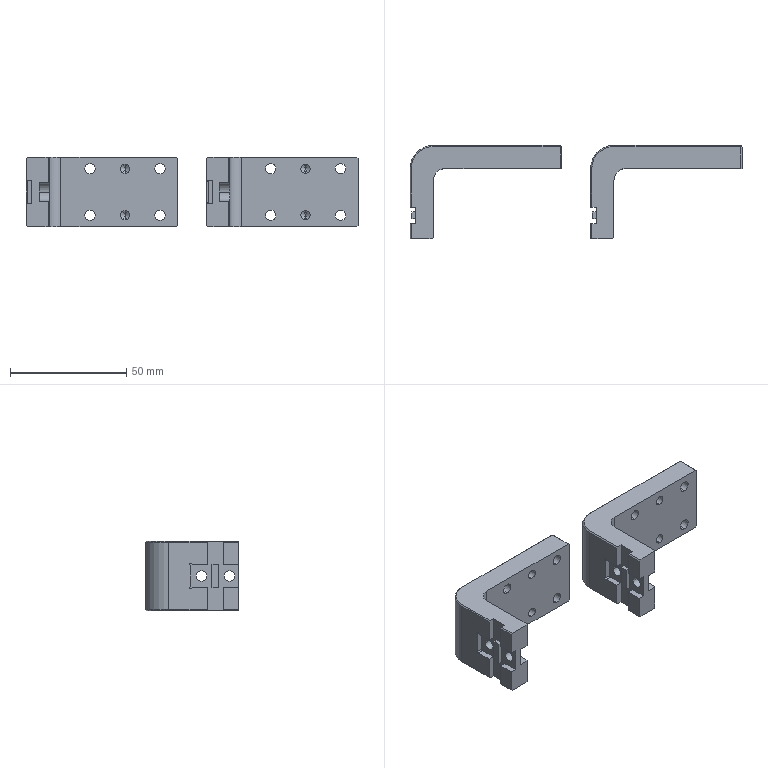Part | 2 solids | 168 faces | box 142.5 x 40 x 30 mm | volume 50240 mm3 | plane 86 | cylinder 66 | cone 16 | commonest cylinder face diameters 4.5 x24 8 x24 4 x8 1 x4 2 x2 10 x2